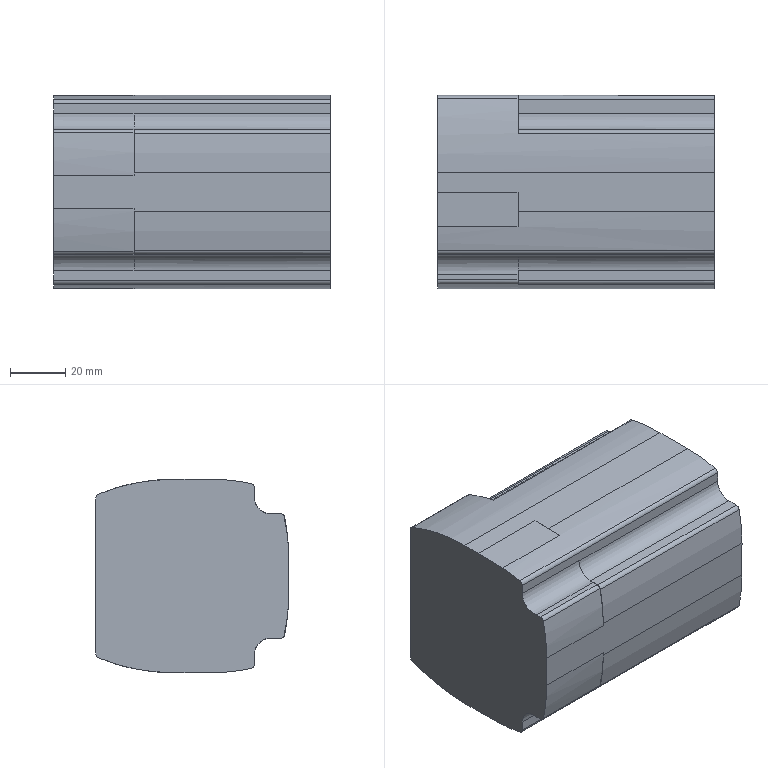Part | STEP file | _BMH070 Lagerschild2A154 | 1 solid | 62 faces | box 100 x 70.1 x 70 mm | volume 431023 mm3 | cylinder 31 | plane 31 | commonest cylinder face diameters 3 x10 140 x8 12 x7 4 x6